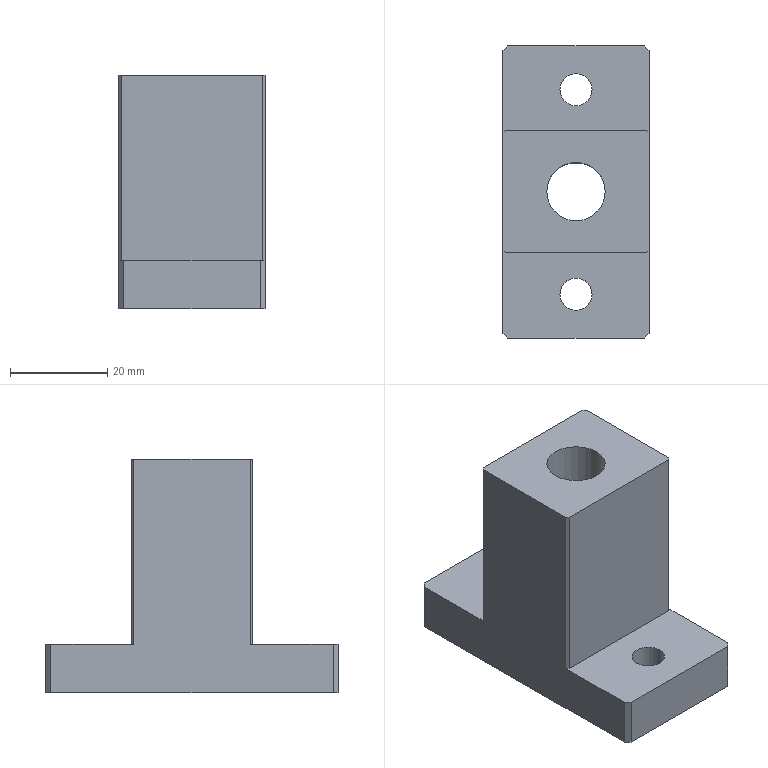Part | NX | 1 solid | 21 faces | box 30 x 60 x 48 mm | volume 40348 mm3 | plane 18 | cylinder 3 | commonest cylinder face diameters 6.6 x2 12 x1
STEP:
#1=CARTESIAN_POINT('',(182.857,139.461,0.));
#2=VERTEX_POINT('',#1);
#3=CARTESIAN_POINT('',(182.357,138.961,0.));
#4=VERTEX_POINT('',#3);
#5=CARTESIAN_POINT('',(182.857,139.461,0.));
#6=DIRECTION('',(-0.7071,-0.7071,0.));
#7=VECTOR('',#6,1000.);
#8=LINE('',#5,#7);
#9=EDGE_CURVE('',#2,#4,#8,.T.);
#10=ORIENTED_EDGE('',*,*,#9,.F.);
#11=CARTESIAN_POINT('',(211.857,139.461,0.));
#12=VERTEX_POINT('',#11);
#13=CARTESIAN_POINT('',(211.857,139.461,0.));
#14=DIRECTION('',(-1.,0.,0.));
#15=VECTOR('',#14,1000.);
#16=LINE('',#13,#15);
#17=EDGE_CURVE('',#12,#2,#16,.T.);
#18=ORIENTED_EDGE('',*,*,#17,.F.);
#19=CARTESIAN_POINT('',(212.357,138.961,0.));
#20=VERTEX_POINT('',#19);
#21=CARTESIAN_POINT('',(212.357,138.961,0.));
#22=DIRECTION('',(-0.7071,0.7071,0.));
#23=VECTOR('',#22,1000.);
#24=LINE('',#21,#23);
#25=EDGE_CURVE('',#20,#12,#24,.T.);
#26=ORIENTED_EDGE('',*,*,#25,.F.);
#27=CARTESIAN_POINT('',(212.357,155.961,0.));
#28=VERTEX_POINT('',#27);
#29=CARTESIAN_POINT('',(212.357,138.961,0.));
#30=DIRECTION('',(0.,1.,0.));
#31=VECTOR('',#30,1000.);
#32=LINE('',#29,#31);
#33=EDGE_CURVE('',#20,#28,#32,.T.);
#34=ORIENTED_EDGE('',*,*,#33,.T.);
#35=CARTESIAN_POINT('',(211.357,156.961,0.));
#36=VERTEX_POINT('',#35);
#37=CARTESIAN_POINT('',(212.357,155.961,0.));
#38=DIRECTION('',(-0.7071,0.7071,0.));
#39=VECTOR('',#38,1000.);
#40=LINE('',#37,#39);
#41=EDGE_CURVE('',#28,#36,#40,.T.);
#42=ORIENTED_EDGE('',*,*,#41,.T.);
#43=CARTESIAN_POINT('',(183.357,156.961,0.));
#44=VERTEX_POINT('',#43);
#45=CARTESIAN_POINT('',(211.357,156.961,0.));
#46=DIRECTION('',(-1.,0.,0.));
#47=VECTOR('',#46,1000.);
#48=LINE('',#45,#47);
#49=EDGE_CURVE('',#36,#44,#48,.T.);
#50=ORIENTED_EDGE('',*,*,#49,.T.);
#51=CARTESIAN_POINT('',(182.357,155.961,0.));
#52=VERTEX_POINT('',#51);
#53=CARTESIAN_POINT('',(183.357,156.961,0.));
#54=DIRECTION('',(-0.7071,-0.7071,0.));
#55=VECTOR('',#54,1000.);
#56=LINE('',#53,#55);
#57=EDGE_CURVE('',#44,#52,#56,.T.);
#58=ORIENTED_EDGE('',*,*,#57,.T.);
#59=CARTESIAN_POINT('',(182.357,114.961,0.));
#60=DIRECTION('',(0.,-1.,0.));
#61=VECTOR('',#60,1000.);
#62=LINE('',#59,#61);
#63=EDGE_CURVE('',#52,#4,#62,.T.);
#64=ORIENTED_EDGE('',*,*,#63,.T.);
#65=EDGE_LOOP('',(#10,#18,#26,#34,#42,#50,#58,#64));
#66=FACE_BOUND('',#65,.T.);
#67=CARTESIAN_POINT('',(200.657,147.961,0.));
#68=VERTEX_POINT('',#67);
#69=CARTESIAN_POINT('',(197.357,147.961,0.));
#70=DIRECTION('',(0.,0.,-1.));
#71=DIRECTION('',(1.,0.,0.));
#72=AXIS2_PLACEMENT_3D('',#69,#70,#71);
#73=CIRCLE('',#72,3.3);
#74=EDGE_CURVE('',#68,#68,#73,.T.);
#75=ORIENTED_EDGE('',*,*,#74,.T.);
#76=EDGE_LOOP('',(#75));
#77=FACE_BOUND('',#76,.T.);
#78=CARTESIAN_POINT('',(0.,0.,0.));
#79=DIRECTION('',(0.,0.,1.));
#80=DIRECTION('',(1.,0.,0.));
#81=AXIS2_PLACEMENT_3D('',#78,#79,#80);
#82=PLANE('',#81);
#83=ADVANCED_FACE('',(#66,#77),#82,.T.);
#84=ORIENTED_EDGE('',*,*,#57,.F.);
#85=CARTESIAN_POINT('',(183.357,156.961,-10.));
#86=VERTEX_POINT('',#85);
#87=CARTESIAN_POINT('',(183.357,156.961,-10.));
#88=DIRECTION('',(0.,0.,1.));
#89=VECTOR('',#88,1000.);
#90=LINE('',#87,#89);
#91=EDGE_CURVE('',#86,#44,#90,.T.);
#92=ORIENTED_EDGE('',*,*,#91,.F.);
#93=CARTESIAN_POINT('',(182.357,155.961,-10.));
#94=VERTEX_POINT('',#93);
#95=CARTESIAN_POINT('',(183.357,156.961,-10.));
#96=DIRECTION('',(-0.7071,-0.7071,0.));
#97=VECTOR('',#96,1000.);
#98=LINE('',#95,#97);
#99=EDGE_CURVE('',#86,#94,#98,.T.);
#100=ORIENTED_EDGE('',*,*,#99,.T.);
#101=CARTESIAN_POINT('',(182.357,155.961,-10.));
#102=DIRECTION('',(0.,0.,1.));
#103=VECTOR('',#102,1000.);
#104=LINE('',#101,#103);
#105=EDGE_CURVE('',#94,#52,#104,.T.);
#106=ORIENTED_EDGE('',*,*,#105,.T.);
#107=EDGE_LOOP('',(#84,#92,#100,#106));
#108=FACE_BOUND('',#107,.T.);
#109=CARTESIAN_POINT('',(183.357,156.961,-10.));
#110=DIRECTION('',(-0.7071,0.7071,0.));
#111=DIRECTION('',(-0.7071,-0.7071,0.));
#112=AXIS2_PLACEMENT_3D('',#109,#110,#111);
#113=PLANE('',#112);
#114=ADVANCED_FACE('',(#108),#113,.T.);
#115=ORIENTED_EDGE('',*,*,#63,.F.);
#116=ORIENTED_EDGE('',*,*,#105,.F.);
#117=CARTESIAN_POINT('',(182.357,97.961,-10.));
#118=VERTEX_POINT('',#117);
#119=CARTESIAN_POINT('',(182.357,155.961,-10.));
#120=DIRECTION('',(0.,-1.,0.));
#121=VECTOR('',#120,1000.);
#122=LINE('',#119,#121);
#123=EDGE_CURVE('',#94,#118,#122,.T.);
#124=ORIENTED_EDGE('',*,*,#123,.T.);
#125=CARTESIAN_POINT('',(182.357,97.961,0.));
#126=VERTEX_POINT('',#125);
#127=CARTESIAN_POINT('',(182.357,97.961,-10.));
#128=DIRECTION('',(0.,0.,1.));
#129=VECTOR('',#128,1000.);
#130=LINE('',#127,#129);
#131=EDGE_CURVE('',#118,#126,#130,.T.);
#132=ORIENTED_EDGE('',*,*,#131,.T.);
#133=CARTESIAN_POINT('',(182.357,114.961,0.));
#134=VERTEX_POINT('',#133);
#135=CARTESIAN_POINT('',(182.357,114.961,0.));
#136=DIRECTION('',(0.,-1.,0.));
#137=VECTOR('',#136,1000.);
#138=LINE('',#135,#137);
#139=EDGE_CURVE('',#134,#126,#138,.T.);
#140=ORIENTED_EDGE('',*,*,#139,.F.);
#141=CARTESIAN_POINT('',(182.357,114.961,38.));
#142=VERTEX_POINT('',#141);
#143=CARTESIAN_POINT('',(182.357,114.961,38.));
#144=DIRECTION('',(0.,0.,-1.));
#145=VECTOR('',#144,1000.);
#146=LINE('',#143,#145);
#147=EDGE_CURVE('',#142,#134,#146,.T.);
#148=ORIENTED_EDGE('',*,*,#147,.F.);
#149=CARTESIAN_POINT('',(182.357,138.961,38.));
#150=VERTEX_POINT('',#149);
#151=CARTESIAN_POINT('',(182.357,138.961,38.));
#152=DIRECTION('',(0.,-1.,0.));
#153=VECTOR('',#152,1000.);
#154=LINE('',#151,#153);
#155=EDGE_CURVE('',#150,#142,#154,.T.);
#156=ORIENTED_EDGE('',*,*,#155,.F.);
#157=CARTESIAN_POINT('',(182.357,138.961,38.));
#158=DIRECTION('',(0.,0.,-1.));
#159=VECTOR('',#158,1000.);
#160=LINE('',#157,#159);
#161=EDGE_CURVE('',#150,#4,#160,.T.);
#162=ORIENTED_EDGE('',*,*,#161,.T.);
#163=EDGE_LOOP('',(#115,#116,#124,#132,#140,#148,#156,#162));
#164=FACE_BOUND('',#163,.T.);
#165=CARTESIAN_POINT('',(182.357,114.961,-10.));
#166=DIRECTION('',(-1.,0.,0.));
#167=DIRECTION('',(0.,0.,1.));
#168=AXIS2_PLACEMENT_3D('',#165,#166,#167);
#169=PLANE('',#168);
#170=ADVANCED_FACE('',(#164),#169,.T.);
#171=CARTESIAN_POINT('',(183.357,96.961,0.));
#172=VERTEX_POINT('',#171);
#173=CARTESIAN_POINT('',(182.357,97.961,0.));
#174=DIRECTION('',(0.7071,-0.7071,0.));
#175=VECTOR('',#174,1000.);
#176=LINE('',#173,#175);
#177=EDGE_CURVE('',#126,#172,#176,.T.);
#178=ORIENTED_EDGE('',*,*,#177,.F.);
#179=ORIENTED_EDGE('',*,*,#131,.F.);
#180=CARTESIAN_POINT('',(183.357,96.961,-10.));
#181=VERTEX_POINT('',#180);
#182=CARTESIAN_POINT('',(182.357,97.961,-10.));
#183=DIRECTION('',(0.7071,-0.7071,0.));
#184=VECTOR('',#183,1000.);
#185=LINE('',#182,#184);
#186=EDGE_CURVE('',#118,#181,#185,.T.);
#187=ORIENTED_EDGE('',*,*,#186,.T.);
#188=CARTESIAN_POINT('',(183.357,96.961,-10.));
#189=DIRECTION('',(0.,0.,1.));
#190=VECTOR('',#189,1000.);
#191=LINE('',#188,#190);
#192=EDGE_CURVE('',#181,#172,#191,.T.);
#193=ORIENTED_EDGE('',*,*,#192,.T.);
#194=EDGE_LOOP('',(#178,#179,#187,#193));
#195=FACE_BOUND('',#194,.T.);
#196=CARTESIAN_POINT('',(182.357,97.961,-10.));
#197=DIRECTION('',(-0.7071,-0.7071,0.));
#198=DIRECTION('',(0.7071,-0.7071,0.));
#199=AXIS2_PLACEMENT_3D('',#196,#197,#198);
#200=PLANE('',#199);
#201=ADVANCED_FACE('',(#195),#200,.T.);
#202=CARTESIAN_POINT('',(211.357,96.961,0.));
#203=VERTEX_POINT('',#202);
#204=CARTESIAN_POINT('',(183.357,96.961,0.));
#205=DIRECTION('',(1.,0.,0.));
#206=VECTOR('',#205,1000.);
#207=LINE('',#204,#206);
#208=EDGE_CURVE('',#172,#203,#207,.T.);
#209=ORIENTED_EDGE('',*,*,#208,.F.);
#210=ORIENTED_EDGE('',*,*,#192,.F.);
#211=CARTESIAN_POINT('',(211.357,96.961,-10.));
#212=VERTEX_POINT('',#211);
#213=CARTESIAN_POINT('',(183.357,96.961,-10.));
#214=DIRECTION('',(1.,0.,0.));
#215=VECTOR('',#214,1000.);
#216=LINE('',#213,#215);
#217=EDGE_CURVE('',#181,#212,#216,.T.);
#218=ORIENTED_EDGE('',*,*,#217,.T.);
#219=CARTESIAN_POINT('',(211.357,96.961,-10.));
#220=DIRECTION('',(0.,0.,1.));
#221=VECTOR('',#220,1000.);
#222=LINE('',#219,#221);
#223=EDGE_CURVE('',#212,#203,#222,.T.);
#224=ORIENTED_EDGE('',*,*,#223,.T.);
#225=EDGE_LOOP('',(#209,#210,#218,#224));
#226=FACE_BOUND('',#225,.T.);
#227=CARTESIAN_POINT('',(183.357,96.961,-10.));
#228=DIRECTION('',(0.,-1.,0.));
#229=DIRECTION('',(0.,0.,-1.));
#230=AXIS2_PLACEMENT_3D('',#227,#228,#229);
#231=PLANE('',#230);
#232=ADVANCED_FACE('',(#226),#231,.T.);
#233=CARTESIAN_POINT('',(212.357,97.961,0.));
#234=VERTEX_POINT('',#233);
#235=CARTESIAN_POINT('',(211.357,96.961,0.));
#236=DIRECTION('',(0.7071,0.7071,0.));
#237=VECTOR('',#236,1000.);
#238=LINE('',#235,#237);
#239=EDGE_CURVE('',#203,#234,#238,.T.);
#240=ORIENTED_EDGE('',*,*,#239,.F.);
#241=ORIENTED_EDGE('',*,*,#223,.F.);
#242=CARTESIAN_POINT('',(212.357,97.961,-10.));
#243=VERTEX_POINT('',#242);
#244=CARTESIAN_POINT('',(211.357,96.961,-10.));
#245=DIRECTION('',(0.7071,0.7071,0.));
#246=VECTOR('',#245,1000.);
#247=LINE('',#244,#246);
#248=EDGE_CURVE('',#212,#243,#247,.T.);
#249=ORIENTED_EDGE('',*,*,#248,.T.);
#250=CARTESIAN_POINT('',(212.357,97.961,-10.));
#251=DIRECTION('',(0.,0.,1.));
#252=VECTOR('',#251,1000.);
#253=LINE('',#250,#252);
#254=EDGE_CURVE('',#243,#234,#253,.T.);
#255=ORIENTED_EDGE('',*,*,#254,.T.);
#256=EDGE_LOOP('',(#240,#241,#249,#255));
#257=FACE_BOUND('',#256,.T.);
#258=CARTESIAN_POINT('',(211.357,96.961,-10.));
#259=DIRECTION('',(0.7071,-0.7071,0.));
#260=DIRECTION('',(0.7071,0.7071,0.));
#261=AXIS2_PLACEMENT_3D('',#258,#259,#260);
#262=PLANE('',#261);
#263=ADVANCED_FACE('',(#257),#262,.T.);
#264=CARTESIAN_POINT('',(212.357,114.961,0.));
#265=VERTEX_POINT('',#264);
#266=CARTESIAN_POINT('',(212.357,138.961,0.));
#267=DIRECTION('',(0.,1.,0.));
#268=VECTOR('',#267,1000.);
#269=LINE('',#266,#268);
#270=EDGE_CURVE('',#234,#265,#269,.T.);
#271=ORIENTED_EDGE('',*,*,#270,.F.);
#272=ORIENTED_EDGE('',*,*,#254,.F.);
#273=CARTESIAN_POINT('',(212.357,155.961,-10.));
#274=VERTEX_POINT('',#273);
#275=CARTESIAN_POINT('',(212.357,97.961,-10.));
#276=DIRECTION('',(0.,1.,0.));
#277=VECTOR('',#276,1000.);
#278=LINE('',#275,#277);
#279=EDGE_CURVE('',#243,#274,#278,.T.);
#280=ORIENTED_EDGE('',*,*,#279,.T.);
#281=CARTESIAN_POINT('',(212.357,155.961,-10.));
#282=DIRECTION('',(0.,0.,1.));
#283=VECTOR('',#282,1000.);
#284=LINE('',#281,#283);
#285=EDGE_CURVE('',#274,#28,#284,.T.);
#286=ORIENTED_EDGE('',*,*,#285,.T.);
#287=ORIENTED_EDGE('',*,*,#33,.F.);
#288=CARTESIAN_POINT('',(212.357,138.961,38.));
#289=VERTEX_POINT('',#288);
#290=CARTESIAN_POINT('',(212.357,138.961,38.));
#291=DIRECTION('',(0.,0.,-1.));
#292=VECTOR('',#291,1000.);
#293=LINE('',#290,#292);
#294=EDGE_CURVE('',#289,#20,#293,.T.);
#295=ORIENTED_EDGE('',*,*,#294,.F.);
#296=CARTESIAN_POINT('',(212.357,114.961,38.));
#297=VERTEX_POINT('',#296);
#298=CARTESIAN_POINT('',(212.357,114.961,38.));
#299=DIRECTION('',(0.,1.,0.));
#300=VECTOR('',#299,1000.);
#301=LINE('',#298,#300);
#302=EDGE_CURVE('',#297,#289,#301,.T.);
#303=ORIENTED_EDGE('',*,*,#302,.F.);
#304=CARTESIAN_POINT('',(212.357,114.961,38.));
#305=DIRECTION('',(0.,0.,-1.));
#306=VECTOR('',#305,1000.);
#307=LINE('',#304,#306);
#308=EDGE_CURVE('',#297,#265,#307,.T.);
#309=ORIENTED_EDGE('',*,*,#308,.T.);
#310=EDGE_LOOP('',(#271,#272,#280,#286,#287,#295,#303,#309));
#311=FACE_BOUND('',#310,.T.);
#312=CARTESIAN_POINT('',(212.357,138.961,-10.));
#313=DIRECTION('',(1.,0.,0.));
#314=DIRECTION('',(0.,0.,-1.));
#315=AXIS2_PLACEMENT_3D('',#312,#313,#314);
#316=PLANE('',#315);
#317=ADVANCED_FACE('',(#311),#316,.T.);
#318=ORIENTED_EDGE('',*,*,#41,.F.);
#319=ORIENTED_EDGE('',*,*,#285,.F.);
#320=CARTESIAN_POINT('',(211.357,156.961,-10.));
#321=VERTEX_POINT('',#320);
#322=CARTESIAN_POINT('',(212.357,155.961,-10.));
#323=DIRECTION('',(-0.7071,0.7071,0.));
#324=VECTOR('',#323,1000.);
#325=LINE('',#322,#324);
#326=EDGE_CURVE('',#274,#321,#325,.T.);
#327=ORIENTED_EDGE('',*,*,#326,.T.);
#328=CARTESIAN_POINT('',(211.357,156.961,-10.));
#329=DIRECTION('',(0.,0.,1.));
#330=VECTOR('',#329,1000.);
#331=LINE('',#328,#330);
#332=EDGE_CURVE('',#321,#36,#331,.T.);
#333=ORIENTED_EDGE('',*,*,#332,.T.);
#334=EDGE_LOOP('',(#318,#319,#327,#333));
#335=FACE_BOUND('',#334,.T.);
#336=CARTESIAN_POINT('',(212.357,155.961,-10.));
#337=DIRECTION('',(0.7071,0.7071,0.));
#338=DIRECTION('',(-0.7071,0.7071,0.));
#339=AXIS2_PLACEMENT_3D('',#336,#337,#338);
#340=PLANE('',#339);
#341=ADVANCED_FACE('',(#335),#340,.T.);
#342=ORIENTED_EDGE('',*,*,#49,.F.);
#343=ORIENTED_EDGE('',*,*,#332,.F.);
#344=CARTESIAN_POINT('',(211.357,156.961,-10.));
#345=DIRECTION('',(-1.,0.,0.));
#346=VECTOR('',#345,1000.);
#347=LINE('',#344,#346);
#348=EDGE_CURVE('',#321,#86,#347,.T.);
#349=ORIENTED_EDGE('',*,*,#348,.T.);
#350=ORIENTED_EDGE('',*,*,#91,.T.);
#351=EDGE_LOOP('',(#342,#343,#349,#350));
#352=FACE_BOUND('',#351,.T.);
#353=CARTESIAN_POINT('',(211.357,156.961,-10.));
#354=DIRECTION('',(0.,1.,0.));
#355=DIRECTION('',(0.,0.,1.));
#356=AXIS2_PLACEMENT_3D('',#353,#354,#355);
#357=PLANE('',#356);
#358=ADVANCED_FACE('',(#352),#357,.T.);
#359=CARTESIAN_POINT('',(203.357,126.961,-10.));
#360=VERTEX_POINT('',#359);
#361=CARTESIAN_POINT('',(197.357,126.961,-10.));
#362=DIRECTION('',(0.,0.,1.));
#363=DIRECTION('',(1.,0.,0.));
#364=AXIS2_PLACEMENT_3D('',#361,#362,#363);
#365=CIRCLE('',#364,6.);
#366=EDGE_CURVE('',#360,#360,#365,.F.);
#367=ORIENTED_EDGE('',*,*,#366,.F.);
#368=EDGE_LOOP('',(#367));
#369=FACE_BOUND('',#368,.T.);
#370=CARTESIAN_POINT('',(200.657,105.961,-10.));
#371=VERTEX_POINT('',#370);
#372=CARTESIAN_POINT('',(197.357,105.961,-10.));
#373=DIRECTION('',(0.,0.,1.));
#374=DIRECTION('',(1.,0.,0.));
#375=AXIS2_PLACEMENT_3D('',#372,#373,#374);
#376=CIRCLE('',#375,3.3);
#377=EDGE_CURVE('',#371,#371,#376,.F.);
#378=ORIENTED_EDGE('',*,*,#377,.F.);
#379=EDGE_LOOP('',(#378));
#380=FACE_BOUND('',#379,.T.);
#381=CARTESIAN_POINT('',(200.657,147.961,-10.));
#382=VERTEX_POINT('',#381);
#383=CARTESIAN_POINT('',(197.357,147.961,-10.));
#384=DIRECTION('',(0.,0.,1.));
#385=DIRECTION('',(1.,0.,0.));
#386=AXIS2_PLACEMENT_3D('',#383,#384,#385);
#387=CIRCLE('',#386,3.3);
#388=EDGE_CURVE('',#382,#382,#387,.F.);
#389=ORIENTED_EDGE('',*,*,#388,.F.);
#390=EDGE_LOOP('',(#389));
#391=FACE_BOUND('',#390,.T.);
#392=ORIENTED_EDGE('',*,*,#99,.F.);
#393=ORIENTED_EDGE('',*,*,#348,.F.);
#394=ORIENTED_EDGE('',*,*,#326,.F.);
#395=ORIENTED_EDGE('',*,*,#279,.F.);
#396=ORIENTED_EDGE('',*,*,#248,.F.);
#397=ORIENTED_EDGE('',*,*,#217,.F.);
#398=ORIENTED_EDGE('',*,*,#186,.F.);
#399=ORIENTED_EDGE('',*,*,#123,.F.);
#400=EDGE_LOOP('',(#392,#393,#394,#395,#396,#397,#398,#399));
#401=FACE_BOUND('',#400,.T.);
#402=CARTESIAN_POINT('',(0.,0.,-10.));
#403=DIRECTION('',(0.,0.,1.));
#404=DIRECTION('',(1.,0.,0.));
#405=AXIS2_PLACEMENT_3D('',#402,#403,#404);
#406=PLANE('',#405);
#407=ADVANCED_FACE('',(#369,#380,#391,#401),#406,.F.);
#408=CARTESIAN_POINT('',(211.857,114.461,0.));
#409=VERTEX_POINT('',#408);
#410=CARTESIAN_POINT('',(211.857,114.461,0.));
#411=DIRECTION('',(0.7071,0.7071,0.));
#412=VECTOR('',#411,1000.);
#413=LINE('',#410,#412);
#414=EDGE_CURVE('',#409,#265,#413,.T.);
#415=ORIENTED_EDGE('',*,*,#414,.F.);
#416=CARTESIAN_POINT('',(182.857,114.461,0.));
#417=VERTEX_POINT('',#416);
#418=CARTESIAN_POINT('',(182.857,114.461,0.));
#419=DIRECTION('',(1.,0.,0.));
#420=VECTOR('',#419,1000.);
#421=LINE('',#418,#420);
#422=EDGE_CURVE('',#417,#409,#421,.T.);
#423=ORIENTED_EDGE('',*,*,#422,.F.);
#424=CARTESIAN_POINT('',(182.357,114.961,0.));
#425=DIRECTION('',(0.7071,-0.7071,0.));
#426=VECTOR('',#425,1000.);
#427=LINE('',#424,#426);
#428=EDGE_CURVE('',#134,#417,#427,.T.);
#429=ORIENTED_EDGE('',*,*,#428,.F.);
#430=ORIENTED_EDGE('',*,*,#139,.T.);
#431=ORIENTED_EDGE('',*,*,#177,.T.);
#432=ORIENTED_EDGE('',*,*,#208,.T.);
#433=ORIENTED_EDGE('',*,*,#239,.T.);
#434=ORIENTED_EDGE('',*,*,#270,.T.);
#435=EDGE_LOOP('',(#415,#423,#429,#430,#431,#432,#433,#434));
#436=FACE_BOUND('',#435,.T.);
#437=CARTESIAN_POINT('',(200.657,105.961,0.));
#438=VERTEX_POINT('',#437);
#439=CARTESIAN_POINT('',(197.357,105.961,0.));
#440=DIRECTION('',(0.,0.,-1.));
#441=DIRECTION('',(1.,0.,0.));
#442=AXIS2_PLACEMENT_3D('',#439,#440,#441);
#443=CIRCLE('',#442,3.3);
#444=EDGE_CURVE('',#438,#438,#443,.T.);
#445=ORIENTED_EDGE('',*,*,#444,.T.);
#446=EDGE_LOOP('',(#445));
#447=FACE_BOUND('',#446,.T.);
#448=CARTESIAN_POINT('',(0.,0.,0.));
#449=DIRECTION('',(0.,0.,1.));
#450=DIRECTION('',(1.,0.,0.));
#451=AXIS2_PLACEMENT_3D('',#448,#449,#450);
#452=PLANE('',#451);
#453=ADVANCED_FACE('',(#436,#447),#452,.T.);
#454=ORIENTED_EDGE('',*,*,#74,.F.);
#455=EDGE_LOOP('',(#454));
#456=FACE_BOUND('',#455,.T.);
#457=ORIENTED_EDGE('',*,*,#388,.T.);
#458=EDGE_LOOP('',(#457));
#459=FACE_BOUND('',#458,.T.);
#460=CARTESIAN_POINT('',(197.357,147.961,-53.));
#461=DIRECTION('',(0.,0.,1.));
#462=DIRECTION('',(1.,0.,0.));
#463=AXIS2_PLACEMENT_3D('',#460,#461,#462);
#464=CYLINDRICAL_SURFACE('',#463,3.3);
#465=ADVANCED_FACE('',(#456,#459),#464,.F.);
#466=ORIENTED_EDGE('',*,*,#444,.F.);
#467=EDGE_LOOP('',(#466));
#468=FACE_BOUND('',#467,.T.);
#469=ORIENTED_EDGE('',*,*,#377,.T.);
#470=EDGE_LOOP('',(#469));
#471=FACE_BOUND('',#470,.T.);
#472=CARTESIAN_POINT('',(197.357,105.961,-53.));
#473=DIRECTION('',(0.,0.,1.));
#474=DIRECTION('',(1.,0.,0.));
#475=AXIS2_PLACEMENT_3D('',#472,#473,#474);
#476=CYLINDRICAL_SURFACE('',#475,3.3);
#477=ADVANCED_FACE('',(#468,#471),#476,.F.);
#478=ORIENTED_EDGE('',*,*,#428,.T.);
#479=CARTESIAN_POINT('',(182.857,114.461,38.));
#480=VERTEX_POINT('',#479);
#481=CARTESIAN_POINT('',(182.857,114.461,38.));
#482=DIRECTION('',(0.,0.,-1.));
#483=VECTOR('',#482,1000.);
#484=LINE('',#481,#483);
#485=EDGE_CURVE('',#480,#417,#484,.T.);
#486=ORIENTED_EDGE('',*,*,#485,.F.);
#487=CARTESIAN_POINT('',(182.357,114.961,38.));
#488=DIRECTION('',(0.7071,-0.7071,0.));
#489=VECTOR('',#488,1000.);
#490=LINE('',#487,#489);
#491=EDGE_CURVE('',#142,#480,#490,.T.);
#492=ORIENTED_EDGE('',*,*,#491,.F.);
#493=ORIENTED_EDGE('',*,*,#147,.T.);
#494=EDGE_LOOP('',(#478,#486,#492,#493));
#495=FACE_BOUND('',#494,.T.);
#496=CARTESIAN_POINT('',(182.357,114.961,38.));
#497=DIRECTION('',(0.7071,0.7071,0.));
#498=DIRECTION('',(-0.7071,0.7071,0.));
#499=AXIS2_PLACEMENT_3D('',#496,#497,#498);
#500=PLANE('',#499);
#501=ADVANCED_FACE('',(#495),#500,.F.);
#502=ORIENTED_EDGE('',*,*,#422,.T.);
#503=CARTESIAN_POINT('',(211.857,114.461,38.));
#504=VERTEX_POINT('',#503);
#505=CARTESIAN_POINT('',(211.857,114.461,38.));
#506=DIRECTION('',(0.,0.,-1.));
#507=VECTOR('',#506,1000.);
#508=LINE('',#505,#507);
#509=EDGE_CURVE('',#504,#409,#508,.T.);
#510=ORIENTED_EDGE('',*,*,#509,.F.);
#511=CARTESIAN_POINT('',(182.857,114.461,38.));
#512=DIRECTION('',(1.,0.,0.));
#513=VECTOR('',#512,1000.);
#514=LINE('',#511,#513);
#515=EDGE_CURVE('',#480,#504,#514,.T.);
#516=ORIENTED_EDGE('',*,*,#515,.F.);
#517=ORIENTED_EDGE('',*,*,#485,.T.);
#518=EDGE_LOOP('',(#502,#510,#516,#517));
#519=FACE_BOUND('',#518,.T.);
#520=CARTESIAN_POINT('',(182.857,114.461,38.));
#521=DIRECTION('',(0.,1.,0.));
#522=DIRECTION('',(0.,0.,1.));
#523=AXIS2_PLACEMENT_3D('',#520,#521,#522);
#524=PLANE('',#523);
#525=ADVANCED_FACE('',(#519),#524,.F.);
#526=ORIENTED_EDGE('',*,*,#414,.T.);
#527=ORIENTED_EDGE('',*,*,#308,.F.);
#528=CARTESIAN_POINT('',(211.857,114.461,38.));
#529=DIRECTION('',(0.7071,0.7071,0.));
#530=VECTOR('',#529,1000.);
#531=LINE('',#528,#530);
#532=EDGE_CURVE('',#504,#297,#531,.T.);
#533=ORIENTED_EDGE('',*,*,#532,.F.);
#534=ORIENTED_EDGE('',*,*,#509,.T.);
#535=EDGE_LOOP('',(#526,#527,#533,#534));
#536=FACE_BOUND('',#535,.T.);
#537=CARTESIAN_POINT('',(211.857,114.461,38.));
#538=DIRECTION('',(-0.7071,0.7071,0.));
#539=DIRECTION('',(-0.7071,-0.7071,0.));
#540=AXIS2_PLACEMENT_3D('',#537,#538,#539);
#541=PLANE('',#540);
#542=ADVANCED_FACE('',(#536),#541,.F.);
#543=ORIENTED_EDGE('',*,*,#25,.T.);
#544=CARTESIAN_POINT('',(211.857,139.461,38.));
#545=VERTEX_POINT('',#544);
#546=CARTESIAN_POINT('',(211.857,139.461,38.));
#547=DIRECTION('',(0.,0.,-1.));
#548=VECTOR('',#547,1000.);
#549=LINE('',#546,#548);
#550=EDGE_CURVE('',#545,#12,#549,.T.);
#551=ORIENTED_EDGE('',*,*,#550,.F.);
#552=CARTESIAN_POINT('',(212.357,138.961,38.));
#553=DIRECTION('',(-0.7071,0.7071,0.));
#554=VECTOR('',#553,1000.);
#555=LINE('',#552,#554);
#556=EDGE_CURVE('',#289,#545,#555,.T.);
#557=ORIENTED_EDGE('',*,*,#556,.F.);
#558=ORIENTED_EDGE('',*,*,#294,.T.);
#559=EDGE_LOOP('',(#543,#551,#557,#558));
#560=FACE_BOUND('',#559,.T.);
#561=CARTESIAN_POINT('',(212.357,138.961,38.));
#562=DIRECTION('',(-0.7071,-0.7071,0.));
#563=DIRECTION('',(0.7071,-0.7071,0.));
#564=AXIS2_PLACEMENT_3D('',#561,#562,#563);
#565=PLANE('',#564);
#566=ADVANCED_FACE('',(#560),#565,.F.);
#567=ORIENTED_EDGE('',*,*,#17,.T.);
#568=CARTESIAN_POINT('',(182.857,139.461,38.));
#569=VERTEX_POINT('',#568);
#570=CARTESIAN_POINT('',(182.857,139.461,38.));
#571=DIRECTION('',(0.,0.,-1.));
#572=VECTOR('',#571,1000.);
#573=LINE('',#570,#572);
#574=EDGE_CURVE('',#569,#2,#573,.T.);
#575=ORIENTED_EDGE('',*,*,#574,.F.);
#576=CARTESIAN_POINT('',(211.857,139.461,38.));
#577=DIRECTION('',(-1.,0.,0.));
#578=VECTOR('',#577,1000.);
#579=LINE('',#576,#578);
#580=EDGE_CURVE('',#545,#569,#579,.T.);
#581=ORIENTED_EDGE('',*,*,#580,.F.);
#582=ORIENTED_EDGE('',*,*,#550,.T.);
#583=EDGE_LOOP('',(#567,#575,#581,#582));
#584=FACE_BOUND('',#583,.T.);
#585=CARTESIAN_POINT('',(211.857,139.461,38.));
#586=DIRECTION('',(0.,-1.,0.));
#587=DIRECTION('',(0.,0.,-1.));
#588=AXIS2_PLACEMENT_3D('',#585,#586,#587);
#589=PLANE('',#588);
#590=ADVANCED_FACE('',(#584),#589,.F.);
#591=ORIENTED_EDGE('',*,*,#9,.T.);
#592=ORIENTED_EDGE('',*,*,#161,.F.);
#593=CARTESIAN_POINT('',(182.857,139.461,38.));
#594=DIRECTION('',(-0.7071,-0.7071,0.));
#595=VECTOR('',#594,1000.);
#596=LINE('',#593,#595);
#597=EDGE_CURVE('',#569,#150,#596,.T.);
#598=ORIENTED_EDGE('',*,*,#597,.F.);
#599=ORIENTED_EDGE('',*,*,#574,.T.);
#600=EDGE_LOOP('',(#591,#592,#598,#599));
#601=FACE_BOUND('',#600,.T.);
#602=CARTESIAN_POINT('',(182.857,139.461,38.));
#603=DIRECTION('',(0.7071,-0.7071,0.));
#604=DIRECTION('',(0.7071,0.7071,0.));
#605=AXIS2_PLACEMENT_3D('',#602,#603,#604);
#606=PLANE('',#605);
#607=ADVANCED_FACE('',(#601),#606,.F.);
#608=CARTESIAN_POINT('',(203.357,126.961,38.));
#609=VERTEX_POINT('',#608);
#610=CARTESIAN_POINT('',(197.357,126.961,38.));
#611=DIRECTION('',(0.,0.,1.));
#612=DIRECTION('',(1.,0.,0.));
#613=AXIS2_PLACEMENT_3D('',#610,#611,#612);
#614=CIRCLE('',#613,6.);
#615=EDGE_CURVE('',#609,#609,#614,.T.);
#616=ORIENTED_EDGE('',*,*,#615,.F.);
#617=EDGE_LOOP('',(#616));
#618=FACE_BOUND('',#617,.T.);
#619=ORIENTED_EDGE('',*,*,#155,.T.);
#620=ORIENTED_EDGE('',*,*,#491,.T.);
#621=ORIENTED_EDGE('',*,*,#515,.T.);
#622=ORIENTED_EDGE('',*,*,#532,.T.);
#623=ORIENTED_EDGE('',*,*,#302,.T.);
#624=ORIENTED_EDGE('',*,*,#556,.T.);
#625=ORIENTED_EDGE('',*,*,#580,.T.);
#626=ORIENTED_EDGE('',*,*,#597,.T.);
#627=EDGE_LOOP('',(#619,#620,#621,#622,#623,#624,#625,#626));
#628=FACE_BOUND('',#627,.T.);
#629=CARTESIAN_POINT('',(0.,0.,38.));
#630=DIRECTION('',(0.,0.,1.));
#631=DIRECTION('',(1.,0.,0.));
#632=AXIS2_PLACEMENT_3D('',#629,#630,#631);
#633=PLANE('',#632);
#634=ADVANCED_FACE('',(#618,#628),#633,.T.);
#635=ORIENTED_EDGE('',*,*,#615,.T.);
#636=EDGE_LOOP('',(#635));
#637=FACE_BOUND('',#636,.T.);
#638=ORIENTED_EDGE('',*,*,#366,.T.);
#639=EDGE_LOOP('',(#638));
#640=FACE_BOUND('',#639,.T.);
#641=CARTESIAN_POINT('',(197.357,126.961,0.));
#642=DIRECTION('',(0.,0.,1.));
#643=DIRECTION('',(1.,0.,0.));
#644=AXIS2_PLACEMENT_3D('',#641,#642,#643);
#645=CYLINDRICAL_SURFACE('',#644,6.);
#646=ADVANCED_FACE('',(#637,#640),#645,.F.);
#647=CLOSED_SHELL('',(#83,#114,#170,#201,#232,#263,#317,#341,#358,#407,#453,#465,#477,#501,#525,#542,#566,#590,#607,#634,#646));
#648=MANIFOLD_SOLID_BREP('',#647);
#649=(LENGTH_UNIT()NAMED_UNIT(*)SI_UNIT(.MILLI.,.METRE.));
#650=UNCERTAINTY_MEASURE_WITH_UNIT(LENGTH_MEASURE(0.00001),#649,'','');
#651=(NAMED_UNIT(*)PLANE_ANGLE_UNIT()SI_UNIT($,.RADIAN.));
#652=(NAMED_UNIT(*)SI_UNIT($,.STERADIAN.)SOLID_ANGLE_UNIT());
#653=(GEOMETRIC_REPRESENTATION_CONTEXT(3)GLOBAL_UNCERTAINTY_ASSIGNED_CONTEXT((#650))GLOBAL_UNIT_ASSIGNED_CONTEXT((#649,#651,#652))REPRESENTATION_CONTEXT('',''));
#654=ADVANCED_BREP_SHAPE_REPRESENTATION('',(#648),#653);